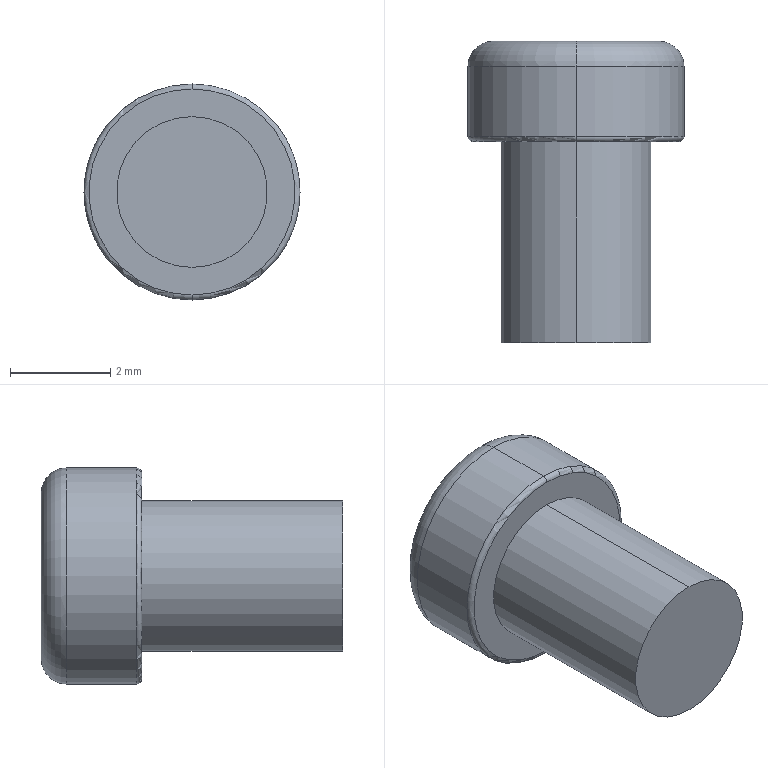Part | SolidWorks | features Fillet 2, ICE 2, Extrusion 1 | 1 solid | 24 faces | box 4.3 x 6 x 4.3 mm | volume 53.843 mm3 | plane 16 | torus 4 | cylinder 4 | commonest cylinder face diameters 3 x2 4.3 x2
STEP:
#1=CARTESIAN_POINT('',(0.,0.,-2.05));
#2=VERTEX_POINT('',#1);
#3=CARTESIAN_POINT('',(0.,0.,2.05));
#4=VERTEX_POINT('',#3);
#5=CARTESIAN_POINT('',(0.,0.,0.));
#6=DIRECTION('',(0.,-1.,0.));
#7=DIRECTION('',(0.,0.,1.));
#8=AXIS2_PLACEMENT_3D('',#5,#6,#7);
#9=CIRCLE('',#8,2.05);
#10=EDGE_CURVE('',#2,#4,#9,.T.);
#11=ORIENTED_EDGE('',*,*,#10,.F.);
#12=CARTESIAN_POINT('',(0.,0.1,-2.15));
#13=VERTEX_POINT('',#12);
#14=CARTESIAN_POINT('',(0.,0.1,-2.05));
#15=DIRECTION('',(1.,0.,0.));
#16=DIRECTION('',(0.,0.,-1.));
#17=AXIS2_PLACEMENT_3D('',#14,#15,#16);
#18=CIRCLE('',#17,0.1);
#19=EDGE_CURVE('',#2,#13,#18,.T.);
#20=ORIENTED_EDGE('',*,*,#19,.T.);
#21=CARTESIAN_POINT('',(0.,0.1,2.15));
#22=VERTEX_POINT('',#21);
#23=CARTESIAN_POINT('',(0.,0.1,0.));
#24=DIRECTION('',(0.,1.,0.));
#25=DIRECTION('',(0.,0.,1.));
#26=AXIS2_PLACEMENT_3D('',#23,#24,#25);
#27=CIRCLE('',#26,2.15);
#28=EDGE_CURVE('',#22,#13,#27,.T.);
#29=ORIENTED_EDGE('',*,*,#28,.F.);
#30=CARTESIAN_POINT('',(0.,0.1,2.05));
#31=DIRECTION('',(-1.,0.,0.));
#32=DIRECTION('',(0.,0.,1.));
#33=AXIS2_PLACEMENT_3D('',#30,#31,#32);
#34=CIRCLE('',#33,0.1);
#35=EDGE_CURVE('',#4,#22,#34,.T.);
#36=ORIENTED_EDGE('',*,*,#35,.F.);
#37=EDGE_LOOP('',(#11,#20,#29,#36));
#38=FACE_OUTER_BOUND('',#37,.T.);
#39=CARTESIAN_POINT('',(0.,0.1,0.));
#40=DIRECTION('',(0.,1.,0.));
#41=DIRECTION('',(0.,0.,1.));
#42=AXIS2_PLACEMENT_3D('',#39,#40,#41);
#43=TOROIDAL_SURFACE('',#42,2.05,0.1);
#44=ADVANCED_FACE('',(#38),#43,.T.);
#45=CARTESIAN_POINT('',(0.,1.5,-2.15));
#46=VERTEX_POINT('',#45);
#47=CARTESIAN_POINT('',(0.,1.5,2.15));
#48=VERTEX_POINT('',#47);
#49=CARTESIAN_POINT('',(0.,1.5,0.));
#50=DIRECTION('',(0.,-1.,0.));
#51=DIRECTION('',(0.,0.,1.));
#52=AXIS2_PLACEMENT_3D('',#49,#50,#51);
#53=CIRCLE('',#52,2.15);
#54=EDGE_CURVE('',#46,#48,#53,.T.);
#55=ORIENTED_EDGE('',*,*,#54,.F.);
#56=CARTESIAN_POINT('',(0.,2.,-1.65));
#57=VERTEX_POINT('',#56);
#58=CARTESIAN_POINT('',(0.,1.5,-1.65));
#59=DIRECTION('',(1.,0.,0.));
#60=DIRECTION('',(0.,0.,-1.));
#61=AXIS2_PLACEMENT_3D('',#58,#59,#60);
#62=CIRCLE('',#61,0.5);
#63=EDGE_CURVE('',#46,#57,#62,.T.);
#64=ORIENTED_EDGE('',*,*,#63,.T.);
#65=CARTESIAN_POINT('',(0.,2.,1.65));
#66=VERTEX_POINT('',#65);
#67=CARTESIAN_POINT('',(0.,2.,0.));
#68=DIRECTION('',(0.,1.,0.));
#69=DIRECTION('',(0.,0.,1.));
#70=AXIS2_PLACEMENT_3D('',#67,#68,#69);
#71=CIRCLE('',#70,1.65);
#72=EDGE_CURVE('',#66,#57,#71,.T.);
#73=ORIENTED_EDGE('',*,*,#72,.F.);
#74=CARTESIAN_POINT('',(0.,1.5,1.65));
#75=DIRECTION('',(-1.,0.,0.));
#76=DIRECTION('',(0.,0.,1.));
#77=AXIS2_PLACEMENT_3D('',#74,#75,#76);
#78=CIRCLE('',#77,0.5);
#79=EDGE_CURVE('',#48,#66,#78,.T.);
#80=ORIENTED_EDGE('',*,*,#79,.F.);
#81=EDGE_LOOP('',(#55,#64,#73,#80));
#82=FACE_OUTER_BOUND('',#81,.T.);
#83=CARTESIAN_POINT('',(0.,1.5,0.));
#84=DIRECTION('',(0.,1.,0.));
#85=DIRECTION('',(0.,0.,1.));
#86=AXIS2_PLACEMENT_3D('',#83,#84,#85);
#87=TOROIDAL_SURFACE('',#86,1.65,0.5);
#88=ADVANCED_FACE('',(#82),#87,.T.);
#89=CARTESIAN_POINT('',(0.,-4.,-1.5));
#90=VERTEX_POINT('',#89);
#91=CARTESIAN_POINT('',(0.,-4.,1.5));
#92=VERTEX_POINT('',#91);
#93=CARTESIAN_POINT('',(0.,-4.,0.));
#94=DIRECTION('',(0.,-1.,0.));
#95=DIRECTION('',(0.,0.,-1.));
#96=AXIS2_PLACEMENT_3D('',#93,#94,#95);
#97=CIRCLE('',#96,1.5);
#98=EDGE_CURVE('',#90,#92,#97,.T.);
#99=ORIENTED_EDGE('',*,*,#98,.F.);
#100=CARTESIAN_POINT('',(0.,0.,-1.5));
#101=VERTEX_POINT('',#100);
#102=CARTESIAN_POINT('',(0.,-4.,-1.5));
#103=DIRECTION('',(0.,1.,0.));
#104=VECTOR('',#103,1000.);
#105=LINE('',#102,#104);
#106=EDGE_CURVE('',#90,#101,#105,.T.);
#107=ORIENTED_EDGE('',*,*,#106,.T.);
#108=CARTESIAN_POINT('',(0.,0.,1.5));
#109=VERTEX_POINT('',#108);
#110=CARTESIAN_POINT('',(0.,0.,0.));
#111=DIRECTION('',(0.,-1.,0.));
#112=DIRECTION('',(0.,0.,1.));
#113=AXIS2_PLACEMENT_3D('',#110,#111,#112);
#114=CIRCLE('',#113,1.5);
#115=EDGE_CURVE('',#101,#109,#114,.T.);
#116=ORIENTED_EDGE('',*,*,#115,.T.);
#117=CARTESIAN_POINT('',(0.,-4.,1.5));
#118=DIRECTION('',(0.,1.,0.));
#119=VECTOR('',#118,1000.);
#120=LINE('',#117,#119);
#121=EDGE_CURVE('',#92,#109,#120,.T.);
#122=ORIENTED_EDGE('',*,*,#121,.F.);
#123=EDGE_LOOP('',(#99,#107,#116,#122));
#124=FACE_OUTER_BOUND('',#123,.T.);
#125=CARTESIAN_POINT('',(0.,-4.,0.));
#126=DIRECTION('',(0.,1.,0.));
#127=DIRECTION('',(0.,0.,1.));
#128=AXIS2_PLACEMENT_3D('',#125,#126,#127);
#129=CYLINDRICAL_SURFACE('',#128,1.5);
#130=ADVANCED_FACE('',(#124),#129,.T.);
#131=ORIENTED_EDGE('',*,*,#54,.T.);
#132=CARTESIAN_POINT('',(0.,2.,2.15));
#133=DIRECTION('',(0.,-1.,0.));
#134=VECTOR('',#133,1000.);
#135=LINE('',#132,#134);
#136=EDGE_CURVE('',#48,#22,#135,.T.);
#137=ORIENTED_EDGE('',*,*,#136,.T.);
#138=ORIENTED_EDGE('',*,*,#28,.T.);
#139=CARTESIAN_POINT('',(0.,2.,-2.15));
#140=DIRECTION('',(0.,-1.,0.));
#141=VECTOR('',#140,1000.);
#142=LINE('',#139,#141);
#143=EDGE_CURVE('',#46,#13,#142,.T.);
#144=ORIENTED_EDGE('',*,*,#143,.F.);
#145=EDGE_LOOP('',(#131,#137,#138,#144));
#146=FACE_OUTER_BOUND('',#145,.T.);
#147=CARTESIAN_POINT('',(0.,2.,0.));
#148=DIRECTION('',(0.,-1.,0.));
#149=DIRECTION('',(0.,0.,-1.));
#150=AXIS2_PLACEMENT_3D('',#147,#148,#149);
#151=CYLINDRICAL_SURFACE('',#150,2.15);
#152=ADVANCED_FACE('',(#146),#151,.T.);
#153=ORIENTED_EDGE('',*,*,#136,.F.);
#154=CARTESIAN_POINT('',(0.,1.5,0.));
#155=DIRECTION('',(0.,-1.,0.));
#156=DIRECTION('',(0.,0.,1.));
#157=AXIS2_PLACEMENT_3D('',#154,#155,#156);
#158=CIRCLE('',#157,2.15);
#159=EDGE_CURVE('',#48,#46,#158,.T.);
#160=ORIENTED_EDGE('',*,*,#159,.T.);
#161=ORIENTED_EDGE('',*,*,#143,.T.);
#162=CARTESIAN_POINT('',(0.,0.1,0.));
#163=DIRECTION('',(0.,1.,0.));
#164=DIRECTION('',(0.,0.,1.));
#165=AXIS2_PLACEMENT_3D('',#162,#163,#164);
#166=CIRCLE('',#165,2.15);
#167=EDGE_CURVE('',#13,#22,#166,.T.);
#168=ORIENTED_EDGE('',*,*,#167,.T.);
#169=EDGE_LOOP('',(#153,#160,#161,#168));
#170=FACE_OUTER_BOUND('',#169,.T.);
#171=CARTESIAN_POINT('',(0.,2.,0.));
#172=DIRECTION('',(0.,-1.,0.));
#173=DIRECTION('',(0.,0.,-1.));
#174=AXIS2_PLACEMENT_3D('',#171,#172,#173);
#175=CYLINDRICAL_SURFACE('',#174,2.15);
#176=ADVANCED_FACE('',(#170),#175,.T.);
#177=CARTESIAN_POINT('',(1.341,2.,0.3));
#178=VERTEX_POINT('',#177);
#179=CARTESIAN_POINT('',(1.341,2.,-0.3));
#180=VERTEX_POINT('',#179);
#181=CARTESIAN_POINT('',(1.341,2.,0.3));
#182=DIRECTION('',(0.,0.,-1.));
#183=VECTOR('',#182,1000.);
#184=LINE('',#181,#183);
#185=EDGE_CURVE('',#178,#180,#184,.T.);
#186=ORIENTED_EDGE('',*,*,#185,.F.);
#187=CARTESIAN_POINT('',(0.2966,2.,0.3));
#188=VERTEX_POINT('',#187);
#189=CARTESIAN_POINT('',(0.2966,2.,0.3));
#190=DIRECTION('',(1.,0.,0.));
#191=VECTOR('',#190,1000.);
#192=LINE('',#189,#191);
#193=EDGE_CURVE('',#188,#178,#192,.T.);
#194=ORIENTED_EDGE('',*,*,#193,.F.);
#195=CARTESIAN_POINT('',(0.2966,2.,1.336));
#196=VERTEX_POINT('',#195);
#197=CARTESIAN_POINT('',(0.2966,2.,1.336));
#198=DIRECTION('',(0.,0.,-1.));
#199=VECTOR('',#198,1000.);
#200=LINE('',#197,#199);
#201=EDGE_CURVE('',#196,#188,#200,.T.);
#202=ORIENTED_EDGE('',*,*,#201,.F.);
#203=CARTESIAN_POINT('',(-0.3034,2.,1.336));
#204=VERTEX_POINT('',#203);
#205=CARTESIAN_POINT('',(-0.3034,2.,1.336));
#206=DIRECTION('',(1.,0.,0.));
#207=VECTOR('',#206,1000.);
#208=LINE('',#205,#207);
#209=EDGE_CURVE('',#204,#196,#208,.T.);
#210=ORIENTED_EDGE('',*,*,#209,.F.);
#211=CARTESIAN_POINT('',(-0.3034,2.,0.3));
#212=VERTEX_POINT('',#211);
#213=CARTESIAN_POINT('',(-0.3034,2.,1.336));
#214=DIRECTION('',(0.,0.,1.));
#215=VECTOR('',#214,1000.);
#216=LINE('',#213,#215);
#217=EDGE_CURVE('',#212,#204,#216,.T.);
#218=ORIENTED_EDGE('',*,*,#217,.F.);
#219=CARTESIAN_POINT('',(-1.341,2.,0.3));
#220=VERTEX_POINT('',#219);
#221=CARTESIAN_POINT('',(-1.341,2.,0.3));
#222=DIRECTION('',(1.,0.,0.));
#223=VECTOR('',#222,1000.);
#224=LINE('',#221,#223);
#225=EDGE_CURVE('',#220,#212,#224,.T.);
#226=ORIENTED_EDGE('',*,*,#225,.F.);
#227=CARTESIAN_POINT('',(-1.341,2.,-0.3));
#228=VERTEX_POINT('',#227);
#229=CARTESIAN_POINT('',(-1.341,2.,0.3));
#230=DIRECTION('',(0.,0.,1.));
#231=VECTOR('',#230,1000.);
#232=LINE('',#229,#231);
#233=EDGE_CURVE('',#228,#220,#232,.T.);
#234=ORIENTED_EDGE('',*,*,#233,.F.);
#235=CARTESIAN_POINT('',(-0.3034,2.,-0.3));
#236=VERTEX_POINT('',#235);
#237=CARTESIAN_POINT('',(-1.341,2.,-0.3));
#238=DIRECTION('',(-1.,0.,0.));
#239=VECTOR('',#238,1000.);
#240=LINE('',#237,#239);
#241=EDGE_CURVE('',#236,#228,#240,.T.);
#242=ORIENTED_EDGE('',*,*,#241,.F.);
#243=CARTESIAN_POINT('',(-0.3034,2.,-1.336));
#244=VERTEX_POINT('',#243);
#245=CARTESIAN_POINT('',(-0.3034,2.,-0.3));
#246=DIRECTION('',(0.,0.,1.));
#247=VECTOR('',#246,1000.);
#248=LINE('',#245,#247);
#249=EDGE_CURVE('',#244,#236,#248,.T.);
#250=ORIENTED_EDGE('',*,*,#249,.F.);
#251=CARTESIAN_POINT('',(0.2966,2.,-1.336));
#252=VERTEX_POINT('',#251);
#253=CARTESIAN_POINT('',(-0.3034,2.,-1.336));
#254=DIRECTION('',(-1.,0.,0.));
#255=VECTOR('',#254,1000.);
#256=LINE('',#253,#255);
#257=EDGE_CURVE('',#252,#244,#256,.T.);
#258=ORIENTED_EDGE('',*,*,#257,.F.);
#259=CARTESIAN_POINT('',(0.2966,2.,-0.3));
#260=VERTEX_POINT('',#259);
#261=CARTESIAN_POINT('',(0.2966,2.,-0.3));
#262=DIRECTION('',(0.,0.,-1.));
#263=VECTOR('',#262,1000.);
#264=LINE('',#261,#263);
#265=EDGE_CURVE('',#260,#252,#264,.T.);
#266=ORIENTED_EDGE('',*,*,#265,.F.);
#267=CARTESIAN_POINT('',(0.2966,2.,-0.3));
#268=DIRECTION('',(-1.,0.,0.));
#269=VECTOR('',#268,1000.);
#270=LINE('',#267,#269);
#271=EDGE_CURVE('',#180,#260,#270,.T.);
#272=ORIENTED_EDGE('',*,*,#271,.F.);
#273=EDGE_LOOP('',(#186,#194,#202,#210,#218,#226,#234,#242,#250,#258,#266,#272));
#274=FACE_BOUND('',#273,.T.);
#275=ORIENTED_EDGE('',*,*,#72,.T.);
#276=CARTESIAN_POINT('',(0.,2.,0.));
#277=DIRECTION('',(0.,1.,0.));
#278=DIRECTION('',(0.,0.,1.));
#279=AXIS2_PLACEMENT_3D('',#276,#277,#278);
#280=CIRCLE('',#279,1.65);
#281=EDGE_CURVE('',#57,#66,#280,.T.);
#282=ORIENTED_EDGE('',*,*,#281,.T.);
#283=EDGE_LOOP('',(#275,#282));
#284=FACE_OUTER_BOUND('',#283,.T.);
#285=CARTESIAN_POINT('',(0.,2.,0.));
#286=DIRECTION('',(0.,1.,0.));
#287=DIRECTION('',(0.,0.,1.));
#288=AXIS2_PLACEMENT_3D('',#285,#286,#287);
#289=PLANE('',#288);
#290=ADVANCED_FACE('',(#274,#284),#289,.T.);
#291=CARTESIAN_POINT('',(0.,0.,0.));
#292=DIRECTION('',(0.,-1.,0.));
#293=DIRECTION('',(0.,0.,1.));
#294=AXIS2_PLACEMENT_3D('',#291,#292,#293);
#295=CIRCLE('',#294,2.05);
#296=EDGE_CURVE('',#4,#2,#295,.T.);
#297=ORIENTED_EDGE('',*,*,#296,.T.);
#298=ORIENTED_EDGE('',*,*,#10,.T.);
#299=EDGE_LOOP('',(#297,#298));
#300=FACE_OUTER_BOUND('',#299,.T.);
#301=CARTESIAN_POINT('',(0.,0.,0.));
#302=DIRECTION('',(0.,-1.,0.));
#303=DIRECTION('',(0.,0.,1.));
#304=AXIS2_PLACEMENT_3D('',#301,#302,#303);
#305=CIRCLE('',#304,1.5);
#306=EDGE_CURVE('',#109,#101,#305,.T.);
#307=ORIENTED_EDGE('',*,*,#306,.F.);
#308=ORIENTED_EDGE('',*,*,#115,.F.);
#309=EDGE_LOOP('',(#307,#308));
#310=FACE_BOUND('',#309,.T.);
#311=CARTESIAN_POINT('',(0.,0.,0.));
#312=DIRECTION('',(0.,1.,0.));
#313=DIRECTION('',(0.,0.,1.));
#314=AXIS2_PLACEMENT_3D('',#311,#312,#313);
#315=PLANE('',#314);
#316=ADVANCED_FACE('',(#300,#310),#315,.F.);
#317=ORIENTED_EDGE('',*,*,#106,.F.);
#318=CARTESIAN_POINT('',(0.,-4.,0.));
#319=DIRECTION('',(0.,-1.,0.));
#320=DIRECTION('',(0.,0.,-1.));
#321=AXIS2_PLACEMENT_3D('',#318,#319,#320);
#322=CIRCLE('',#321,1.5);
#323=EDGE_CURVE('',#92,#90,#322,.T.);
#324=ORIENTED_EDGE('',*,*,#323,.F.);
#325=ORIENTED_EDGE('',*,*,#121,.T.);
#326=ORIENTED_EDGE('',*,*,#306,.T.);
#327=EDGE_LOOP('',(#317,#324,#325,#326));
#328=FACE_OUTER_BOUND('',#327,.T.);
#329=CARTESIAN_POINT('',(0.,-4.,0.));
#330=DIRECTION('',(0.,1.,0.));
#331=DIRECTION('',(0.,0.,1.));
#332=AXIS2_PLACEMENT_3D('',#329,#330,#331);
#333=CYLINDRICAL_SURFACE('',#332,1.5);
#334=ADVANCED_FACE('',(#328),#333,.T.);
#335=ORIENTED_EDGE('',*,*,#323,.T.);
#336=ORIENTED_EDGE('',*,*,#98,.T.);
#337=EDGE_LOOP('',(#335,#336));
#338=FACE_OUTER_BOUND('',#337,.T.);
#339=CARTESIAN_POINT('',(0.,-4.,0.));
#340=DIRECTION('',(0.,-1.,0.));
#341=DIRECTION('',(0.,0.,-1.));
#342=AXIS2_PLACEMENT_3D('',#339,#340,#341);
#343=PLANE('',#342);
#344=ADVANCED_FACE('',(#338),#343,.T.);
#345=ORIENTED_EDGE('',*,*,#63,.F.);
#346=ORIENTED_EDGE('',*,*,#159,.F.);
#347=ORIENTED_EDGE('',*,*,#79,.T.);
#348=ORIENTED_EDGE('',*,*,#281,.F.);
#349=EDGE_LOOP('',(#345,#346,#347,#348));
#350=FACE_OUTER_BOUND('',#349,.T.);
#351=CARTESIAN_POINT('',(0.,1.5,0.));
#352=DIRECTION('',(0.,1.,0.));
#353=DIRECTION('',(0.,0.,1.));
#354=AXIS2_PLACEMENT_3D('',#351,#352,#353);
#355=TOROIDAL_SURFACE('',#354,1.65,0.5);
#356=ADVANCED_FACE('',(#350),#355,.T.);
#357=ORIENTED_EDGE('',*,*,#19,.F.);
#358=ORIENTED_EDGE('',*,*,#296,.F.);
#359=ORIENTED_EDGE('',*,*,#35,.T.);
#360=ORIENTED_EDGE('',*,*,#167,.F.);
#361=EDGE_LOOP('',(#357,#358,#359,#360));
#362=FACE_OUTER_BOUND('',#361,.T.);
#363=CARTESIAN_POINT('',(0.,0.1,0.));
#364=DIRECTION('',(0.,1.,0.));
#365=DIRECTION('',(0.,0.,1.));
#366=AXIS2_PLACEMENT_3D('',#363,#364,#365);
#367=TOROIDAL_SURFACE('',#366,2.05,0.1);
#368=ADVANCED_FACE('',(#362),#367,.T.);
#369=ORIENTED_EDGE('',*,*,#185,.T.);
#370=CARTESIAN_POINT('',(1.323,1.,-0.2825));
#371=VERTEX_POINT('',#370);
#372=CARTESIAN_POINT('',(1.34,1.99,-0.2998));
#373=DIRECTION('',(0.01745,0.9997,-0.01745));
#374=VECTOR('',#373,1000.);
#375=LINE('',#372,#374);
#376=EDGE_CURVE('',#371,#180,#375,.T.);
#377=ORIENTED_EDGE('',*,*,#376,.F.);
#378=CARTESIAN_POINT('',(1.323,1.,0.2825));
#379=VERTEX_POINT('',#378);
#380=CARTESIAN_POINT('',(1.323,1.,0.3));
#381=DIRECTION('',(0.,0.,-1.));
#382=VECTOR('',#381,1000.);
#383=LINE('',#380,#382);
#384=EDGE_CURVE('',#379,#371,#383,.T.);
#385=ORIENTED_EDGE('',*,*,#384,.F.);
#386=CARTESIAN_POINT('',(1.34,1.982,0.2997));
#387=DIRECTION('',(0.01745,0.9997,0.01745));
#388=VECTOR('',#387,1000.);
#389=LINE('',#386,#388);
#390=EDGE_CURVE('',#379,#178,#389,.T.);
#391=ORIENTED_EDGE('',*,*,#390,.T.);
#392=EDGE_LOOP('',(#369,#377,#385,#391));
#393=FACE_OUTER_BOUND('',#392,.T.);
#394=CARTESIAN_POINT('',(1.341,2.,0.3));
#395=DIRECTION('',(0.9998,-0.01745,0.));
#396=DIRECTION('',(0.01745,0.9998,0.));
#397=AXIS2_PLACEMENT_3D('',#394,#395,#396);
#398=PLANE('',#397);
#399=ADVANCED_FACE('',(#393),#398,.F.);
#400=ORIENTED_EDGE('',*,*,#193,.T.);
#401=ORIENTED_EDGE('',*,*,#390,.F.);
#402=CARTESIAN_POINT('',(0.2791,1.,0.2825));
#403=VERTEX_POINT('',#402);
#404=CARTESIAN_POINT('',(0.2966,1.,0.2825));
#405=DIRECTION('',(1.,0.,0.));
#406=VECTOR('',#405,1000.);
#407=LINE('',#404,#406);
#408=EDGE_CURVE('',#403,#379,#407,.T.);
#409=ORIENTED_EDGE('',*,*,#408,.F.);
#410=CARTESIAN_POINT('',(0.2966,2.,0.3));
#411=DIRECTION('',(0.01745,0.9997,0.01745));
#412=VECTOR('',#411,1000.);
#413=LINE('',#410,#412);
#414=EDGE_CURVE('',#403,#188,#413,.T.);
#415=ORIENTED_EDGE('',*,*,#414,.T.);
#416=EDGE_LOOP('',(#400,#401,#409,#415));
#417=FACE_OUTER_BOUND('',#416,.T.);
#418=CARTESIAN_POINT('',(0.2966,2.,0.3));
#419=DIRECTION('',(0.,-0.01745,0.9998));
#420=DIRECTION('',(0.,-0.9998,-0.01745));
#421=AXIS2_PLACEMENT_3D('',#418,#419,#420);
#422=PLANE('',#421);
#423=ADVANCED_FACE('',(#417),#422,.F.);
#424=ORIENTED_EDGE('',*,*,#201,.T.);
#425=ORIENTED_EDGE('',*,*,#414,.F.);
#426=CARTESIAN_POINT('',(0.2791,1.,1.319));
#427=VERTEX_POINT('',#426);
#428=CARTESIAN_POINT('',(0.2791,1.,1.336));
#429=DIRECTION('',(0.,0.,-1.));
#430=VECTOR('',#429,1000.);
#431=LINE('',#428,#430);
#432=EDGE_CURVE('',#427,#403,#431,.T.);
#433=ORIENTED_EDGE('',*,*,#432,.F.);
#434=CARTESIAN_POINT('',(0.2964,1.99,1.336));
#435=DIRECTION('',(0.01745,0.9997,0.01745));
#436=VECTOR('',#435,1000.);
#437=LINE('',#434,#436);
#438=EDGE_CURVE('',#427,#196,#437,.T.);
#439=ORIENTED_EDGE('',*,*,#438,.T.);
#440=EDGE_LOOP('',(#424,#425,#433,#439));
#441=FACE_OUTER_BOUND('',#440,.T.);
#442=CARTESIAN_POINT('',(0.2966,2.,1.336));
#443=DIRECTION('',(0.9998,-0.01745,0.));
#444=DIRECTION('',(0.01745,0.9998,0.));
#445=AXIS2_PLACEMENT_3D('',#442,#443,#444);
#446=PLANE('',#445);
#447=ADVANCED_FACE('',(#441),#446,.F.);
#448=ORIENTED_EDGE('',*,*,#209,.T.);
#449=ORIENTED_EDGE('',*,*,#438,.F.);
#450=CARTESIAN_POINT('',(-0.286,1.,1.319));
#451=VERTEX_POINT('',#450);
#452=CARTESIAN_POINT('',(-0.3034,1.,1.319));
#453=DIRECTION('',(1.,0.,0.));
#454=VECTOR('',#453,1000.);
#455=LINE('',#452,#454);
#456=EDGE_CURVE('',#451,#427,#455,.T.);
#457=ORIENTED_EDGE('',*,*,#456,.F.);
#458=CARTESIAN_POINT('',(-0.3034,2.,1.336));
#459=DIRECTION('',(-0.01745,0.9997,0.01745));
#460=VECTOR('',#459,1000.);
#461=LINE('',#458,#460);
#462=EDGE_CURVE('',#451,#204,#461,.T.);
#463=ORIENTED_EDGE('',*,*,#462,.T.);
#464=EDGE_LOOP('',(#448,#449,#457,#463));
#465=FACE_OUTER_BOUND('',#464,.T.);
#466=CARTESIAN_POINT('',(-0.3034,2.,1.336));
#467=DIRECTION('',(0.,-0.01745,0.9998));
#468=DIRECTION('',(0.,-0.9998,-0.01745));
#469=AXIS2_PLACEMENT_3D('',#466,#467,#468);
#470=PLANE('',#469);
#471=ADVANCED_FACE('',(#465),#470,.F.);
#472=ORIENTED_EDGE('',*,*,#217,.T.);
#473=ORIENTED_EDGE('',*,*,#462,.F.);
#474=CARTESIAN_POINT('',(-0.286,1.,0.2825));
#475=VERTEX_POINT('',#474);
#476=CARTESIAN_POINT('',(-0.286,1.,1.336));
#477=DIRECTION('',(0.,0.,1.));
#478=VECTOR('',#477,1000.);
#479=LINE('',#476,#478);
#480=EDGE_CURVE('',#475,#451,#479,.T.);
#481=ORIENTED_EDGE('',*,*,#480,.F.);
#482=CARTESIAN_POINT('',(-0.3037,2.018,0.3003));
#483=DIRECTION('',(-0.01745,0.9997,0.01745));
#484=VECTOR('',#483,1000.);
#485=LINE('',#482,#484);
#486=EDGE_CURVE('',#475,#212,#485,.T.);
#487=ORIENTED_EDGE('',*,*,#486,.T.);
#488=EDGE_LOOP('',(#472,#473,#481,#487));
#489=FACE_OUTER_BOUND('',#488,.T.);
#490=CARTESIAN_POINT('',(-0.3034,2.,1.336));
#491=DIRECTION('',(-0.9998,-0.01745,0.));
#492=DIRECTION('',(0.01745,-0.9998,0.));
#493=AXIS2_PLACEMENT_3D('',#490,#491,#492);
#494=PLANE('',#493);
#495=ADVANCED_FACE('',(#489),#494,.F.);
#496=ORIENTED_EDGE('',*,*,#225,.T.);
#497=ORIENTED_EDGE('',*,*,#486,.F.);
#498=CARTESIAN_POINT('',(-1.323,1.,0.2825));
#499=VERTEX_POINT('',#498);
#500=CARTESIAN_POINT('',(-1.341,1.,0.2825));
#501=DIRECTION('',(1.,0.,0.));
#502=VECTOR('',#501,1000.);
#503=LINE('',#500,#502);
#504=EDGE_CURVE('',#499,#475,#503,.T.);
#505=ORIENTED_EDGE('',*,*,#504,.F.);
#506=CARTESIAN_POINT('',(-1.341,2.,0.3));
#507=DIRECTION('',(-0.01745,0.9997,0.01745));
#508=VECTOR('',#507,1000.);
#509=LINE('',#506,#508);
#510=EDGE_CURVE('',#499,#220,#509,.T.);
#511=ORIENTED_EDGE('',*,*,#510,.T.);
#512=EDGE_LOOP('',(#496,#497,#505,#511));
#513=FACE_OUTER_BOUND('',#512,.T.);
#514=CARTESIAN_POINT('',(-1.341,2.,0.3));
#515=DIRECTION('',(0.,-0.01745,0.9998));
#516=DIRECTION('',(0.,-0.9998,-0.01745));
#517=AXIS2_PLACEMENT_3D('',#514,#515,#516);
#518=PLANE('',#517);
#519=ADVANCED_FACE('',(#513),#518,.F.);
#520=ORIENTED_EDGE('',*,*,#233,.T.);
#521=ORIENTED_EDGE('',*,*,#510,.F.);
#522=CARTESIAN_POINT('',(-1.323,1.,-0.2825));
#523=VERTEX_POINT('',#522);
#524=CARTESIAN_POINT('',(-1.323,1.,0.3));
#525=DIRECTION('',(0.,0.,1.));
#526=VECTOR('',#525,1000.);
#527=LINE('',#524,#526);
#528=EDGE_CURVE('',#523,#499,#527,.T.);
#529=ORIENTED_EDGE('',*,*,#528,.F.);
#530=CARTESIAN_POINT('',(-1.341,2.,-0.3));
#531=DIRECTION('',(-0.01745,0.9997,-0.01745));
#532=VECTOR('',#531,1000.);
#533=LINE('',#530,#532);
#534=EDGE_CURVE('',#523,#228,#533,.T.);
#535=ORIENTED_EDGE('',*,*,#534,.T.);
#536=EDGE_LOOP('',(#520,#521,#529,#535));
#537=FACE_OUTER_BOUND('',#536,.T.);
#538=CARTESIAN_POINT('',(-1.341,2.,0.3));
#539=DIRECTION('',(-0.9998,-0.01745,0.));
#540=DIRECTION('',(0.01745,-0.9998,0.));
#541=AXIS2_PLACEMENT_3D('',#538,#539,#540);
#542=PLANE('',#541);
#543=ADVANCED_FACE('',(#537),#542,.F.);
#544=ORIENTED_EDGE('',*,*,#241,.T.);
#545=ORIENTED_EDGE('',*,*,#534,.F.);
#546=CARTESIAN_POINT('',(-0.286,1.,-0.2825));
#547=VERTEX_POINT('',#546);
#548=CARTESIAN_POINT('',(-1.341,1.,-0.2825));
#549=DIRECTION('',(-1.,0.,0.));
#550=VECTOR('',#549,1000.);
#551=LINE('',#548,#550);
#552=EDGE_CURVE('',#547,#523,#551,.T.);
#553=ORIENTED_EDGE('',*,*,#552,.F.);
#554=CARTESIAN_POINT('',(-0.3037,2.018,-0.3003));
#555=DIRECTION('',(-0.01745,0.9997,-0.01745));
#556=VECTOR('',#555,1000.);
#557=LINE('',#554,#556);
#558=EDGE_CURVE('',#547,#236,#557,.T.);
#559=ORIENTED_EDGE('',*,*,#558,.T.);
#560=EDGE_LOOP('',(#544,#545,#553,#559));
#561=FACE_OUTER_BOUND('',#560,.T.);
#562=CARTESIAN_POINT('',(-1.341,2.,-0.3));
#563=DIRECTION('',(0.,-0.01745,-0.9998));
#564=DIRECTION('',(0.,0.9998,-0.01745));
#565=AXIS2_PLACEMENT_3D('',#562,#563,#564);
#566=PLANE('',#565);
#567=ADVANCED_FACE('',(#561),#566,.F.);
#568=ORIENTED_EDGE('',*,*,#249,.T.);
#569=ORIENTED_EDGE('',*,*,#558,.F.);
#570=CARTESIAN_POINT('',(-0.286,1.,-1.319));
#571=VERTEX_POINT('',#570);
#572=CARTESIAN_POINT('',(-0.286,1.,-0.3));
#573=DIRECTION('',(0.,0.,1.));
#574=VECTOR('',#573,1000.);
#575=LINE('',#572,#574);
#576=EDGE_CURVE('',#571,#547,#575,.T.);
#577=ORIENTED_EDGE('',*,*,#576,.F.);
#578=CARTESIAN_POINT('',(-0.3034,2.,-1.336));
#579=DIRECTION('',(-0.01745,0.9997,-0.01745));
#580=VECTOR('',#579,1000.);
#581=LINE('',#578,#580);
#582=EDGE_CURVE('',#571,#244,#581,.T.);
#583=ORIENTED_EDGE('',*,*,#582,.T.);
#584=EDGE_LOOP('',(#568,#569,#577,#583));
#585=FACE_OUTER_BOUND('',#584,.T.);
#586=CARTESIAN_POINT('',(-0.3034,2.,-0.3));
#587=DIRECTION('',(-0.9998,-0.01745,0.));
#588=DIRECTION('',(0.01745,-0.9998,0.));
#589=AXIS2_PLACEMENT_3D('',#586,#587,#588);
#590=PLANE('',#589);
#591=ADVANCED_FACE('',(#585),#590,.F.);
#592=ORIENTED_EDGE('',*,*,#257,.T.);
#593=ORIENTED_EDGE('',*,*,#582,.F.);
#594=CARTESIAN_POINT('',(0.2791,1.,-1.319));
#595=VERTEX_POINT('',#594);
#596=CARTESIAN_POINT('',(-0.3034,1.,-1.319));
#597=DIRECTION('',(-1.,0.,0.));
#598=VECTOR('',#597,1000.);
#599=LINE('',#596,#598);
#600=EDGE_CURVE('',#595,#571,#599,.T.);
#601=ORIENTED_EDGE('',*,*,#600,.F.);
#602=CARTESIAN_POINT('',(0.2963,1.982,-1.336));
#603=DIRECTION('',(0.01745,0.9997,-0.01745));
#604=VECTOR('',#603,1000.);
#605=LINE('',#602,#604);
#606=EDGE_CURVE('',#595,#252,#605,.T.);
#607=ORIENTED_EDGE('',*,*,#606,.T.);
#608=EDGE_LOOP('',(#592,#593,#601,#607));
#609=FACE_OUTER_BOUND('',#608,.T.);
#610=CARTESIAN_POINT('',(-0.3034,2.,-1.336));
#611=DIRECTION('',(0.,-0.01745,-0.9998));
#612=DIRECTION('',(0.,0.9998,-0.01745));
#613=AXIS2_PLACEMENT_3D('',#610,#611,#612);
#614=PLANE('',#613);
#615=ADVANCED_FACE('',(#609),#614,.F.);
#616=ORIENTED_EDGE('',*,*,#265,.T.);
#617=ORIENTED_EDGE('',*,*,#606,.F.);
#618=CARTESIAN_POINT('',(0.2791,1.,-0.2825));
#619=VERTEX_POINT('',#618);
#620=CARTESIAN_POINT('',(0.2791,1.,-0.3));
#621=DIRECTION('',(0.,0.,-1.));
#622=VECTOR('',#621,1000.);
#623=LINE('',#620,#622);
#624=EDGE_CURVE('',#619,#595,#623,.T.);
#625=ORIENTED_EDGE('',*,*,#624,.F.);
#626=CARTESIAN_POINT('',(0.2966,2.,-0.3));
#627=DIRECTION('',(0.01745,0.9997,-0.01745));
#628=VECTOR('',#627,1000.);
#629=LINE('',#626,#628);
#630=EDGE_CURVE('',#619,#260,#629,.T.);
#631=ORIENTED_EDGE('',*,*,#630,.T.);
#632=EDGE_LOOP('',(#616,#617,#625,#631));
#633=FACE_OUTER_BOUND('',#632,.T.);
#634=CARTESIAN_POINT('',(0.2966,2.,-0.3));
#635=DIRECTION('',(0.9998,-0.01745,0.));
#636=DIRECTION('',(0.01745,0.9998,0.));
#637=AXIS2_PLACEMENT_3D('',#634,#635,#636);
#638=PLANE('',#637);
#639=ADVANCED_FACE('',(#633),#638,.F.);
#640=ORIENTED_EDGE('',*,*,#271,.T.);
#641=ORIENTED_EDGE('',*,*,#630,.F.);
#642=CARTESIAN_POINT('',(0.2966,1.,-0.2825));
#643=DIRECTION('',(-1.,0.,0.));
#644=VECTOR('',#643,1000.);
#645=LINE('',#642,#644);
#646=EDGE_CURVE('',#371,#619,#645,.T.);
#647=ORIENTED_EDGE('',*,*,#646,.F.);
#648=ORIENTED_EDGE('',*,*,#376,.T.);
#649=EDGE_LOOP('',(#640,#641,#647,#648));
#650=FACE_OUTER_BOUND('',#649,.T.);
#651=CARTESIAN_POINT('',(0.2966,2.,-0.3));
#652=DIRECTION('',(0.,-0.01745,-0.9998));
#653=DIRECTION('',(0.,0.9998,-0.01745));
#654=AXIS2_PLACEMENT_3D('',#651,#652,#653);
#655=PLANE('',#654);
#656=ADVANCED_FACE('',(#650),#655,.F.);
#657=ORIENTED_EDGE('',*,*,#384,.T.);
#658=ORIENTED_EDGE('',*,*,#646,.T.);
#659=ORIENTED_EDGE('',*,*,#624,.T.);
#660=ORIENTED_EDGE('',*,*,#600,.T.);
#661=ORIENTED_EDGE('',*,*,#576,.T.);
#662=ORIENTED_EDGE('',*,*,#552,.T.);
#663=ORIENTED_EDGE('',*,*,#528,.T.);
#664=ORIENTED_EDGE('',*,*,#504,.T.);
#665=ORIENTED_EDGE('',*,*,#480,.T.);
#666=ORIENTED_EDGE('',*,*,#456,.T.);
#667=ORIENTED_EDGE('',*,*,#432,.T.);
#668=ORIENTED_EDGE('',*,*,#408,.T.);
#669=EDGE_LOOP('',(#657,#658,#659,#660,#661,#662,#663,#664,#665,#666,#667,#668));
#670=FACE_OUTER_BOUND('',#669,.T.);
#671=CARTESIAN_POINT('',(0.,1.,0.));
#672=DIRECTION('',(0.,-1.,0.));
#673=DIRECTION('',(0.,0.,-1.));
#674=AXIS2_PLACEMENT_3D('',#671,#672,#673);
#675=PLANE('',#674);
#676=ADVANCED_FACE('',(#670),#675,.F.);
#677=CLOSED_SHELL('',(#44,#88,#130,#152,#176,#290,#316,#334,#344,#356,#368,#399,#423,#447,#471,#495,#519,#543,#567,#591,#615,#639,#656,#676));
#678=MANIFOLD_SOLID_BREP('',#677);
#679=CARTESIAN_POINT('',(0.,0.,0.));
#680=DIRECTION('',(0.,0.,1.));
#681=DIRECTION('',(1.,0.,0.));
#682=AXIS2_PLACEMENT_3D('',#679,#680,#681);
#683=(LENGTH_UNIT()NAMED_UNIT(*)SI_UNIT(.MILLI.,.METRE.));
#684=UNCERTAINTY_MEASURE_WITH_UNIT(LENGTH_MEASURE(0.00001),#683,'','');
#685=(NAMED_UNIT(*)PLANE_ANGLE_UNIT()SI_UNIT($,.RADIAN.));
#686=(NAMED_UNIT(*)SI_UNIT($,.STERADIAN.)SOLID_ANGLE_UNIT());
#687=(GEOMETRIC_REPRESENTATION_CONTEXT(3)GLOBAL_UNCERTAINTY_ASSIGNED_CONTEXT((#684))GLOBAL_UNIT_ASSIGNED_CONTEXT((#683,#685,#686))REPRESENTATION_CONTEXT('',''));
#688=ADVANCED_BREP_SHAPE_REPRESENTATION('',(#678,#682),#687);